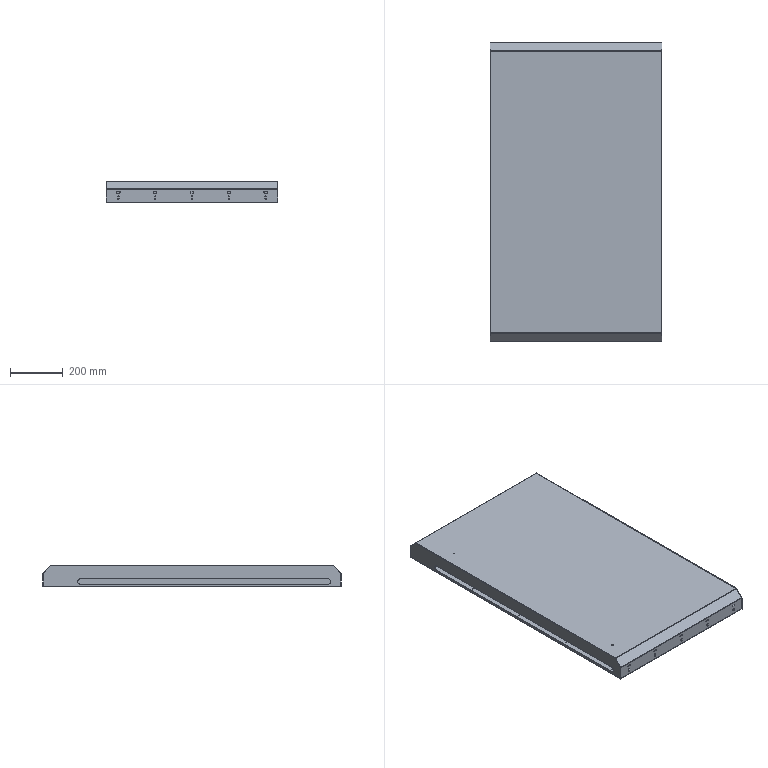Part | NX | features BREP 4 | 4 solids | 155 faces | box 650 x 1132 x 82 mm | volume 1741335 mm3 | plane 80 | cylinder 75 | commonest cylinder face diameters 6 x29 4.2 x28 4 x12 7 x4 20 x2